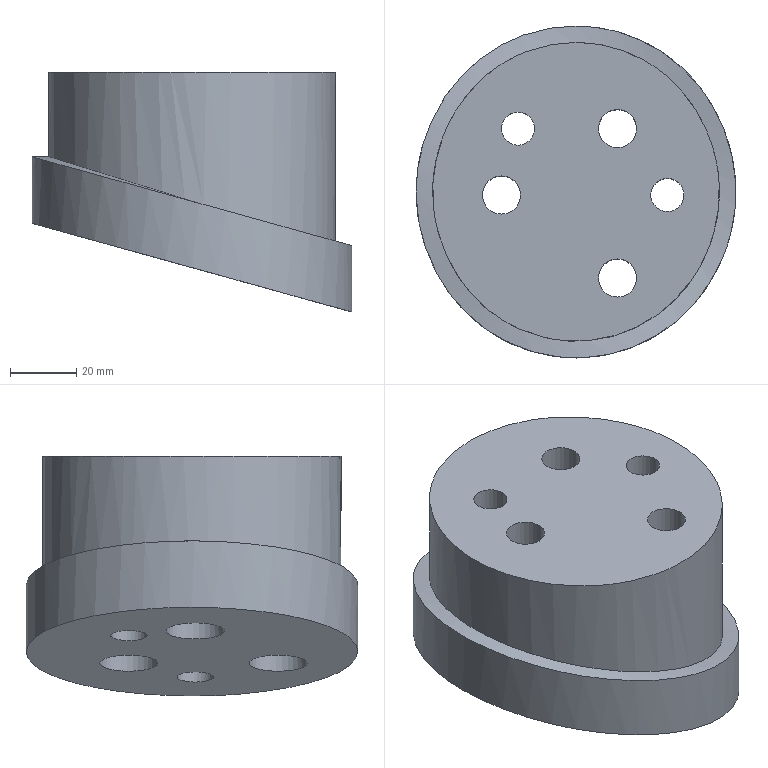Part | NX | features solid 2 | 1 solid | 20 faces | box 96.417 x 100.002 x 72.312 mm | volume 347913 mm3 | cylinder 10 | plane 6 | spline 4 | commonest cylinder face diameters 11.5 x3 17.5 x3 10 x2 11 x2